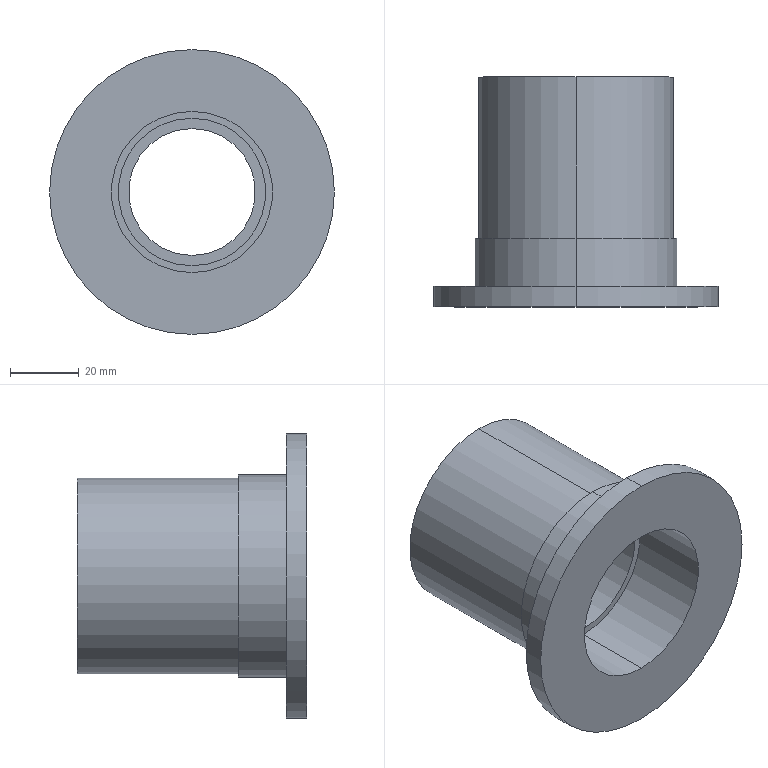Part | SolidWorks | features ICE 1, Revolution 1 | 1 solid | 24 faces | box 83 x 67 x 83 mm | volume 83007 mm3 | cylinder 16 | plane 8 | commonest cylinder face diameters 47 x4 37 x2 43 x2 49 x2 57 x2 59 x2
STEP:
#1=CARTESIAN_POINT('',(0.,67.,24.5));
#2=VERTEX_POINT('',#1);
#3=CARTESIAN_POINT('',(0.,67.,-24.5));
#4=VERTEX_POINT('',#3);
#5=CARTESIAN_POINT('',(0.,67.,0.));
#6=DIRECTION('',(0.,-1.,0.));
#7=DIRECTION('',(0.,0.,-1.));
#8=AXIS2_PLACEMENT_3D('',#5,#6,#7);
#9=CIRCLE('',#8,24.5);
#10=EDGE_CURVE('',#2,#4,#9,.T.);
#11=ORIENTED_EDGE('',*,*,#10,.F.);
#12=CARTESIAN_POINT('',(0.,57.,24.5));
#13=VERTEX_POINT('',#12);
#14=CARTESIAN_POINT('',(0.,0.,24.5));
#15=DIRECTION('',(0.,-1.,0.));
#16=VECTOR('',#15,1000.);
#17=LINE('',#14,#16);
#18=EDGE_CURVE('',#2,#13,#17,.T.);
#19=ORIENTED_EDGE('',*,*,#18,.T.);
#20=CARTESIAN_POINT('',(0.,57.,-24.5));
#21=VERTEX_POINT('',#20);
#22=CARTESIAN_POINT('',(0.,57.,0.));
#23=DIRECTION('',(0.,-1.,0.));
#24=DIRECTION('',(0.,0.,-1.));
#25=AXIS2_PLACEMENT_3D('',#22,#23,#24);
#26=CIRCLE('',#25,24.5);
#27=EDGE_CURVE('',#13,#21,#26,.T.);
#28=ORIENTED_EDGE('',*,*,#27,.T.);
#29=CARTESIAN_POINT('',(0.,0.,-24.5));
#30=DIRECTION('',(0.,-1.,0.));
#31=VECTOR('',#30,1000.);
#32=LINE('',#29,#31);
#33=EDGE_CURVE('',#4,#21,#32,.T.);
#34=ORIENTED_EDGE('',*,*,#33,.F.);
#35=EDGE_LOOP('',(#11,#19,#28,#34));
#36=FACE_OUTER_BOUND('',#35,.T.);
#37=CARTESIAN_POINT('',(0.,0.,0.));
#38=DIRECTION('',(0.,-1.,0.));
#39=DIRECTION('',(0.,0.,-1.));
#40=AXIS2_PLACEMENT_3D('',#37,#38,#39);
#41=CYLINDRICAL_SURFACE('',#40,24.5);
#42=ADVANCED_FACE('',(#36),#41,.F.);
#43=CARTESIAN_POINT('',(0.,67.,-28.5));
#44=VERTEX_POINT('',#43);
#45=CARTESIAN_POINT('',(0.,67.,28.5));
#46=VERTEX_POINT('',#45);
#47=CARTESIAN_POINT('',(0.,67.,0.));
#48=DIRECTION('',(0.,-1.,0.));
#49=DIRECTION('',(0.,0.,-1.));
#50=AXIS2_PLACEMENT_3D('',#47,#48,#49);
#51=CIRCLE('',#50,28.5);
#52=EDGE_CURVE('',#44,#46,#51,.T.);
#53=ORIENTED_EDGE('',*,*,#52,.T.);
#54=CARTESIAN_POINT('',(0.,20.,28.5));
#55=VERTEX_POINT('',#54);
#56=CARTESIAN_POINT('',(0.,0.,28.5));
#57=DIRECTION('',(0.,-1.,0.));
#58=VECTOR('',#57,1000.);
#59=LINE('',#56,#58);
#60=EDGE_CURVE('',#46,#55,#59,.T.);
#61=ORIENTED_EDGE('',*,*,#60,.T.);
#62=CARTESIAN_POINT('',(0.,20.,-28.5));
#63=VERTEX_POINT('',#62);
#64=CARTESIAN_POINT('',(0.,20.,0.));
#65=DIRECTION('',(0.,-1.,0.));
#66=DIRECTION('',(0.,0.,-1.));
#67=AXIS2_PLACEMENT_3D('',#64,#65,#66);
#68=CIRCLE('',#67,28.5);
#69=EDGE_CURVE('',#63,#55,#68,.T.);
#70=ORIENTED_EDGE('',*,*,#69,.F.);
#71=CARTESIAN_POINT('',(0.,0.,-28.5));
#72=DIRECTION('',(0.,-1.,0.));
#73=VECTOR('',#72,1000.);
#74=LINE('',#71,#73);
#75=EDGE_CURVE('',#44,#63,#74,.T.);
#76=ORIENTED_EDGE('',*,*,#75,.F.);
#77=EDGE_LOOP('',(#53,#61,#70,#76));
#78=FACE_OUTER_BOUND('',#77,.T.);
#79=CARTESIAN_POINT('',(0.,0.,0.));
#80=DIRECTION('',(0.,-1.,0.));
#81=DIRECTION('',(0.,0.,-1.));
#82=AXIS2_PLACEMENT_3D('',#79,#80,#81);
#83=CYLINDRICAL_SURFACE('',#82,28.5);
#84=ADVANCED_FACE('',(#78),#83,.T.);
#85=CARTESIAN_POINT('',(0.,20.,-29.5));
#86=VERTEX_POINT('',#85);
#87=CARTESIAN_POINT('',(0.,20.,29.5));
#88=VERTEX_POINT('',#87);
#89=CARTESIAN_POINT('',(0.,20.,0.));
#90=DIRECTION('',(0.,-1.,0.));
#91=DIRECTION('',(0.,0.,-1.));
#92=AXIS2_PLACEMENT_3D('',#89,#90,#91);
#93=CIRCLE('',#92,29.5);
#94=EDGE_CURVE('',#86,#88,#93,.T.);
#95=ORIENTED_EDGE('',*,*,#94,.T.);
#96=CARTESIAN_POINT('',(0.,6.,29.5));
#97=VERTEX_POINT('',#96);
#98=CARTESIAN_POINT('',(0.,0.,29.5));
#99=DIRECTION('',(0.,-1.,0.));
#100=VECTOR('',#99,1000.);
#101=LINE('',#98,#100);
#102=EDGE_CURVE('',#88,#97,#101,.T.);
#103=ORIENTED_EDGE('',*,*,#102,.T.);
#104=CARTESIAN_POINT('',(0.,6.,-29.5));
#105=VERTEX_POINT('',#104);
#106=CARTESIAN_POINT('',(0.,6.,0.));
#107=DIRECTION('',(0.,-1.,0.));
#108=DIRECTION('',(0.,0.,-1.));
#109=AXIS2_PLACEMENT_3D('',#106,#107,#108);
#110=CIRCLE('',#109,29.5);
#111=EDGE_CURVE('',#105,#97,#110,.T.);
#112=ORIENTED_EDGE('',*,*,#111,.F.);
#113=CARTESIAN_POINT('',(0.,0.,-29.5));
#114=DIRECTION('',(0.,-1.,0.));
#115=VECTOR('',#114,1000.);
#116=LINE('',#113,#115);
#117=EDGE_CURVE('',#86,#105,#116,.T.);
#118=ORIENTED_EDGE('',*,*,#117,.F.);
#119=EDGE_LOOP('',(#95,#103,#112,#118));
#120=FACE_OUTER_BOUND('',#119,.T.);
#121=CARTESIAN_POINT('',(0.,0.,0.));
#122=DIRECTION('',(0.,-1.,0.));
#123=DIRECTION('',(0.,0.,-1.));
#124=AXIS2_PLACEMENT_3D('',#121,#122,#123);
#125=CYLINDRICAL_SURFACE('',#124,29.5);
#126=ADVANCED_FACE('',(#120),#125,.T.);
#127=CARTESIAN_POINT('',(0.,6.,-41.5));
#128=VERTEX_POINT('',#127);
#129=CARTESIAN_POINT('',(0.,6.,41.5));
#130=VERTEX_POINT('',#129);
#131=CARTESIAN_POINT('',(0.,6.,0.));
#132=DIRECTION('',(0.,-1.,0.));
#133=DIRECTION('',(0.,0.,-1.));
#134=AXIS2_PLACEMENT_3D('',#131,#132,#133);
#135=CIRCLE('',#134,41.5);
#136=EDGE_CURVE('',#128,#130,#135,.T.);
#137=ORIENTED_EDGE('',*,*,#136,.T.);
#138=CARTESIAN_POINT('',(0.,0.,41.5));
#139=VERTEX_POINT('',#138);
#140=CARTESIAN_POINT('',(0.,0.,41.5));
#141=DIRECTION('',(0.,-1.,0.));
#142=VECTOR('',#141,1000.);
#143=LINE('',#140,#142);
#144=EDGE_CURVE('',#130,#139,#143,.T.);
#145=ORIENTED_EDGE('',*,*,#144,.T.);
#146=CARTESIAN_POINT('',(0.,0.,-41.5));
#147=VERTEX_POINT('',#146);
#148=CARTESIAN_POINT('',(0.,0.,0.));
#149=DIRECTION('',(0.,-1.,0.));
#150=DIRECTION('',(0.,0.,-1.));
#151=AXIS2_PLACEMENT_3D('',#148,#149,#150);
#152=CIRCLE('',#151,41.5);
#153=EDGE_CURVE('',#147,#139,#152,.T.);
#154=ORIENTED_EDGE('',*,*,#153,.F.);
#155=CARTESIAN_POINT('',(0.,0.,-41.5));
#156=DIRECTION('',(0.,-1.,0.));
#157=VECTOR('',#156,1000.);
#158=LINE('',#155,#157);
#159=EDGE_CURVE('',#128,#147,#158,.T.);
#160=ORIENTED_EDGE('',*,*,#159,.F.);
#161=EDGE_LOOP('',(#137,#145,#154,#160));
#162=FACE_OUTER_BOUND('',#161,.T.);
#163=CARTESIAN_POINT('',(0.,0.,0.));
#164=DIRECTION('',(0.,-1.,0.));
#165=DIRECTION('',(0.,0.,-1.));
#166=AXIS2_PLACEMENT_3D('',#163,#164,#165);
#167=CYLINDRICAL_SURFACE('',#166,41.5);
#168=ADVANCED_FACE('',(#162),#167,.T.);
#169=CARTESIAN_POINT('',(0.,24.,23.5));
#170=VERTEX_POINT('',#169);
#171=CARTESIAN_POINT('',(0.,24.,-23.5));
#172=VERTEX_POINT('',#171);
#173=CARTESIAN_POINT('',(0.,24.,0.));
#174=DIRECTION('',(0.,-1.,0.));
#175=DIRECTION('',(0.,0.,-1.));
#176=AXIS2_PLACEMENT_3D('',#173,#174,#175);
#177=CIRCLE('',#176,23.5);
#178=EDGE_CURVE('',#170,#172,#177,.T.);
#179=ORIENTED_EDGE('',*,*,#178,.F.);
#180=CARTESIAN_POINT('',(0.,0.,23.5));
#181=VERTEX_POINT('',#180);
#182=CARTESIAN_POINT('',(0.,0.,23.5));
#183=DIRECTION('',(0.,-1.,0.));
#184=VECTOR('',#183,1000.);
#185=LINE('',#182,#184);
#186=EDGE_CURVE('',#170,#181,#185,.T.);
#187=ORIENTED_EDGE('',*,*,#186,.T.);
#188=CARTESIAN_POINT('',(0.,0.,-23.5));
#189=VERTEX_POINT('',#188);
#190=CARTESIAN_POINT('',(0.,0.,0.));
#191=DIRECTION('',(0.,-1.,0.));
#192=DIRECTION('',(0.,0.,-1.));
#193=AXIS2_PLACEMENT_3D('',#190,#191,#192);
#194=CIRCLE('',#193,23.5);
#195=EDGE_CURVE('',#181,#189,#194,.T.);
#196=ORIENTED_EDGE('',*,*,#195,.T.);
#197=CARTESIAN_POINT('',(0.,0.,-23.5));
#198=DIRECTION('',(0.,-1.,0.));
#199=VECTOR('',#198,1000.);
#200=LINE('',#197,#199);
#201=EDGE_CURVE('',#172,#189,#200,.T.);
#202=ORIENTED_EDGE('',*,*,#201,.F.);
#203=EDGE_LOOP('',(#179,#187,#196,#202));
#204=FACE_OUTER_BOUND('',#203,.T.);
#205=CARTESIAN_POINT('',(0.,0.,0.));
#206=DIRECTION('',(0.,-1.,0.));
#207=DIRECTION('',(0.,0.,-1.));
#208=AXIS2_PLACEMENT_3D('',#205,#206,#207);
#209=CYLINDRICAL_SURFACE('',#208,23.5);
#210=ADVANCED_FACE('',(#204),#209,.F.);
#211=CARTESIAN_POINT('',(0.,48.,21.5));
#212=VERTEX_POINT('',#211);
#213=CARTESIAN_POINT('',(0.,48.,-21.5));
#214=VERTEX_POINT('',#213);
#215=CARTESIAN_POINT('',(0.,48.,0.));
#216=DIRECTION('',(0.,-1.,0.));
#217=DIRECTION('',(0.,0.,-1.));
#218=AXIS2_PLACEMENT_3D('',#215,#216,#217);
#219=CIRCLE('',#218,21.5);
#220=EDGE_CURVE('',#212,#214,#219,.T.);
#221=ORIENTED_EDGE('',*,*,#220,.F.);
#222=CARTESIAN_POINT('',(0.,24.,21.5));
#223=VERTEX_POINT('',#222);
#224=CARTESIAN_POINT('',(0.,0.,21.5));
#225=DIRECTION('',(0.,-1.,0.));
#226=VECTOR('',#225,1000.);
#227=LINE('',#224,#226);
#228=EDGE_CURVE('',#212,#223,#227,.T.);
#229=ORIENTED_EDGE('',*,*,#228,.T.);
#230=CARTESIAN_POINT('',(0.,24.,-21.5));
#231=VERTEX_POINT('',#230);
#232=CARTESIAN_POINT('',(0.,24.,0.));
#233=DIRECTION('',(0.,-1.,0.));
#234=DIRECTION('',(0.,0.,-1.));
#235=AXIS2_PLACEMENT_3D('',#232,#233,#234);
#236=CIRCLE('',#235,21.5);
#237=EDGE_CURVE('',#223,#231,#236,.T.);
#238=ORIENTED_EDGE('',*,*,#237,.T.);
#239=CARTESIAN_POINT('',(0.,0.,-21.5));
#240=DIRECTION('',(0.,-1.,0.));
#241=VECTOR('',#240,1000.);
#242=LINE('',#239,#241);
#243=EDGE_CURVE('',#214,#231,#242,.T.);
#244=ORIENTED_EDGE('',*,*,#243,.F.);
#245=EDGE_LOOP('',(#221,#229,#238,#244));
#246=FACE_OUTER_BOUND('',#245,.T.);
#247=CARTESIAN_POINT('',(0.,0.,0.));
#248=DIRECTION('',(0.,-1.,0.));
#249=DIRECTION('',(0.,0.,-1.));
#250=AXIS2_PLACEMENT_3D('',#247,#248,#249);
#251=CYLINDRICAL_SURFACE('',#250,21.5);
#252=ADVANCED_FACE('',(#246),#251,.F.);
#253=CARTESIAN_POINT('',(0.,53.,18.5));
#254=VERTEX_POINT('',#253);
#255=CARTESIAN_POINT('',(0.,53.,-18.5));
#256=VERTEX_POINT('',#255);
#257=CARTESIAN_POINT('',(0.,53.,0.));
#258=DIRECTION('',(0.,-1.,0.));
#259=DIRECTION('',(0.,0.,-1.));
#260=AXIS2_PLACEMENT_3D('',#257,#258,#259);
#261=CIRCLE('',#260,18.5);
#262=EDGE_CURVE('',#254,#256,#261,.T.);
#263=ORIENTED_EDGE('',*,*,#262,.F.);
#264=CARTESIAN_POINT('',(0.,48.,18.5));
#265=VERTEX_POINT('',#264);
#266=CARTESIAN_POINT('',(0.,0.,18.5));
#267=DIRECTION('',(0.,-1.,0.));
#268=VECTOR('',#267,1000.);
#269=LINE('',#266,#268);
#270=EDGE_CURVE('',#254,#265,#269,.T.);
#271=ORIENTED_EDGE('',*,*,#270,.T.);
#272=CARTESIAN_POINT('',(0.,48.,-18.5));
#273=VERTEX_POINT('',#272);
#274=CARTESIAN_POINT('',(0.,48.,0.));
#275=DIRECTION('',(0.,-1.,0.));
#276=DIRECTION('',(0.,0.,-1.));
#277=AXIS2_PLACEMENT_3D('',#274,#275,#276);
#278=CIRCLE('',#277,18.5);
#279=EDGE_CURVE('',#265,#273,#278,.T.);
#280=ORIENTED_EDGE('',*,*,#279,.T.);
#281=CARTESIAN_POINT('',(0.,0.,-18.5));
#282=DIRECTION('',(0.,-1.,0.));
#283=VECTOR('',#282,1000.);
#284=LINE('',#281,#283);
#285=EDGE_CURVE('',#256,#273,#284,.T.);
#286=ORIENTED_EDGE('',*,*,#285,.F.);
#287=EDGE_LOOP('',(#263,#271,#280,#286));
#288=FACE_OUTER_BOUND('',#287,.T.);
#289=CARTESIAN_POINT('',(0.,0.,0.));
#290=DIRECTION('',(0.,-1.,0.));
#291=DIRECTION('',(0.,0.,-1.));
#292=AXIS2_PLACEMENT_3D('',#289,#290,#291);
#293=CYLINDRICAL_SURFACE('',#292,18.5);
#294=ADVANCED_FACE('',(#288),#293,.F.);
#295=CARTESIAN_POINT('',(0.,57.,23.5));
#296=VERTEX_POINT('',#295);
#297=CARTESIAN_POINT('',(0.,57.,-23.5));
#298=VERTEX_POINT('',#297);
#299=CARTESIAN_POINT('',(0.,57.,0.));
#300=DIRECTION('',(0.,-1.,0.));
#301=DIRECTION('',(0.,0.,-1.));
#302=AXIS2_PLACEMENT_3D('',#299,#300,#301);
#303=CIRCLE('',#302,23.5);
#304=EDGE_CURVE('',#296,#298,#303,.T.);
#305=ORIENTED_EDGE('',*,*,#304,.F.);
#306=CARTESIAN_POINT('',(0.,53.,23.5));
#307=VERTEX_POINT('',#306);
#308=CARTESIAN_POINT('',(0.,0.,23.5));
#309=DIRECTION('',(0.,-1.,0.));
#310=VECTOR('',#309,1000.);
#311=LINE('',#308,#310);
#312=EDGE_CURVE('',#296,#307,#311,.T.);
#313=ORIENTED_EDGE('',*,*,#312,.T.);
#314=CARTESIAN_POINT('',(0.,53.,-23.5));
#315=VERTEX_POINT('',#314);
#316=CARTESIAN_POINT('',(0.,53.,0.));
#317=DIRECTION('',(0.,-1.,0.));
#318=DIRECTION('',(0.,0.,-1.));
#319=AXIS2_PLACEMENT_3D('',#316,#317,#318);
#320=CIRCLE('',#319,23.5);
#321=EDGE_CURVE('',#307,#315,#320,.T.);
#322=ORIENTED_EDGE('',*,*,#321,.T.);
#323=CARTESIAN_POINT('',(0.,0.,-23.5));
#324=DIRECTION('',(0.,-1.,0.));
#325=VECTOR('',#324,1000.);
#326=LINE('',#323,#325);
#327=EDGE_CURVE('',#298,#315,#326,.T.);
#328=ORIENTED_EDGE('',*,*,#327,.F.);
#329=EDGE_LOOP('',(#305,#313,#322,#328));
#330=FACE_OUTER_BOUND('',#329,.T.);
#331=CARTESIAN_POINT('',(0.,0.,0.));
#332=DIRECTION('',(0.,-1.,0.));
#333=DIRECTION('',(0.,0.,-1.));
#334=AXIS2_PLACEMENT_3D('',#331,#332,#333);
#335=CYLINDRICAL_SURFACE('',#334,23.5);
#336=ADVANCED_FACE('',(#330),#335,.F.);
#337=CARTESIAN_POINT('',(0.,57.,0.));
#338=DIRECTION('',(0.,-1.,0.));
#339=DIRECTION('',(0.,0.,-1.));
#340=AXIS2_PLACEMENT_3D('',#337,#338,#339);
#341=CIRCLE('',#340,24.5);
#342=EDGE_CURVE('',#21,#13,#341,.T.);
#343=ORIENTED_EDGE('',*,*,#342,.F.);
#344=ORIENTED_EDGE('',*,*,#27,.F.);
#345=EDGE_LOOP('',(#343,#344));
#346=FACE_OUTER_BOUND('',#345,.T.);
#347=CARTESIAN_POINT('',(0.,57.,0.));
#348=DIRECTION('',(0.,-1.,0.));
#349=DIRECTION('',(0.,0.,-1.));
#350=AXIS2_PLACEMENT_3D('',#347,#348,#349);
#351=CIRCLE('',#350,23.5);
#352=EDGE_CURVE('',#298,#296,#351,.T.);
#353=ORIENTED_EDGE('',*,*,#352,.T.);
#354=ORIENTED_EDGE('',*,*,#304,.T.);
#355=EDGE_LOOP('',(#353,#354));
#356=FACE_BOUND('',#355,.T.);
#357=CARTESIAN_POINT('',(-23.5,57.,0.));
#358=DIRECTION('',(0.,-1.,0.));
#359=DIRECTION('',(0.,0.,-1.));
#360=AXIS2_PLACEMENT_3D('',#357,#358,#359);
#361=PLANE('',#360);
#362=ADVANCED_FACE('',(#346,#356),#361,.F.);
#363=ORIENTED_EDGE('',*,*,#312,.F.);
#364=ORIENTED_EDGE('',*,*,#352,.F.);
#365=ORIENTED_EDGE('',*,*,#327,.T.);
#366=CARTESIAN_POINT('',(0.,53.,0.));
#367=DIRECTION('',(0.,-1.,0.));
#368=DIRECTION('',(0.,0.,-1.));
#369=AXIS2_PLACEMENT_3D('',#366,#367,#368);
#370=CIRCLE('',#369,23.5);
#371=EDGE_CURVE('',#315,#307,#370,.T.);
#372=ORIENTED_EDGE('',*,*,#371,.T.);
#373=EDGE_LOOP('',(#363,#364,#365,#372));
#374=FACE_OUTER_BOUND('',#373,.T.);
#375=CARTESIAN_POINT('',(0.,0.,0.));
#376=DIRECTION('',(0.,-1.,0.));
#377=DIRECTION('',(0.,0.,-1.));
#378=AXIS2_PLACEMENT_3D('',#375,#376,#377);
#379=CYLINDRICAL_SURFACE('',#378,23.5);
#380=ADVANCED_FACE('',(#374),#379,.F.);
#381=ORIENTED_EDGE('',*,*,#371,.F.);
#382=ORIENTED_EDGE('',*,*,#321,.F.);
#383=EDGE_LOOP('',(#381,#382));
#384=FACE_OUTER_BOUND('',#383,.T.);
#385=CARTESIAN_POINT('',(0.,53.,0.));
#386=DIRECTION('',(0.,-1.,0.));
#387=DIRECTION('',(0.,0.,-1.));
#388=AXIS2_PLACEMENT_3D('',#385,#386,#387);
#389=CIRCLE('',#388,18.5);
#390=EDGE_CURVE('',#256,#254,#389,.T.);
#391=ORIENTED_EDGE('',*,*,#390,.T.);
#392=ORIENTED_EDGE('',*,*,#262,.T.);
#393=EDGE_LOOP('',(#391,#392));
#394=FACE_BOUND('',#393,.T.);
#395=CARTESIAN_POINT('',(-23.5,53.,0.));
#396=DIRECTION('',(0.,-1.,0.));
#397=DIRECTION('',(0.,0.,-1.));
#398=AXIS2_PLACEMENT_3D('',#395,#396,#397);
#399=PLANE('',#398);
#400=ADVANCED_FACE('',(#384,#394),#399,.F.);
#401=ORIENTED_EDGE('',*,*,#270,.F.);
#402=ORIENTED_EDGE('',*,*,#390,.F.);
#403=ORIENTED_EDGE('',*,*,#285,.T.);
#404=CARTESIAN_POINT('',(0.,48.,0.));
#405=DIRECTION('',(0.,-1.,0.));
#406=DIRECTION('',(0.,0.,-1.));
#407=AXIS2_PLACEMENT_3D('',#404,#405,#406);
#408=CIRCLE('',#407,18.5);
#409=EDGE_CURVE('',#273,#265,#408,.T.);
#410=ORIENTED_EDGE('',*,*,#409,.T.);
#411=EDGE_LOOP('',(#401,#402,#403,#410));
#412=FACE_OUTER_BOUND('',#411,.T.);
#413=CARTESIAN_POINT('',(0.,0.,0.));
#414=DIRECTION('',(0.,-1.,0.));
#415=DIRECTION('',(0.,0.,-1.));
#416=AXIS2_PLACEMENT_3D('',#413,#414,#415);
#417=CYLINDRICAL_SURFACE('',#416,18.5);
#418=ADVANCED_FACE('',(#412),#417,.F.);
#419=ORIENTED_EDGE('',*,*,#409,.F.);
#420=ORIENTED_EDGE('',*,*,#279,.F.);
#421=EDGE_LOOP('',(#419,#420));
#422=FACE_BOUND('',#421,.T.);
#423=CARTESIAN_POINT('',(0.,48.,0.));
#424=DIRECTION('',(0.,-1.,0.));
#425=DIRECTION('',(0.,0.,-1.));
#426=AXIS2_PLACEMENT_3D('',#423,#424,#425);
#427=CIRCLE('',#426,21.5);
#428=EDGE_CURVE('',#214,#212,#427,.T.);
#429=ORIENTED_EDGE('',*,*,#428,.T.);
#430=ORIENTED_EDGE('',*,*,#220,.T.);
#431=EDGE_LOOP('',(#429,#430));
#432=FACE_OUTER_BOUND('',#431,.T.);
#433=CARTESIAN_POINT('',(-18.5,48.,0.));
#434=DIRECTION('',(0.,1.,0.));
#435=DIRECTION('',(0.,0.,1.));
#436=AXIS2_PLACEMENT_3D('',#433,#434,#435);
#437=PLANE('',#436);
#438=ADVANCED_FACE('',(#422,#432),#437,.F.);
#439=ORIENTED_EDGE('',*,*,#228,.F.);
#440=ORIENTED_EDGE('',*,*,#428,.F.);
#441=ORIENTED_EDGE('',*,*,#243,.T.);
#442=CARTESIAN_POINT('',(0.,24.,0.));
#443=DIRECTION('',(0.,-1.,0.));
#444=DIRECTION('',(0.,0.,-1.));
#445=AXIS2_PLACEMENT_3D('',#442,#443,#444);
#446=CIRCLE('',#445,21.5);
#447=EDGE_CURVE('',#231,#223,#446,.T.);
#448=ORIENTED_EDGE('',*,*,#447,.T.);
#449=EDGE_LOOP('',(#439,#440,#441,#448));
#450=FACE_OUTER_BOUND('',#449,.T.);
#451=CARTESIAN_POINT('',(0.,0.,0.));
#452=DIRECTION('',(0.,-1.,0.));
#453=DIRECTION('',(0.,0.,-1.));
#454=AXIS2_PLACEMENT_3D('',#451,#452,#453);
#455=CYLINDRICAL_SURFACE('',#454,21.5);
#456=ADVANCED_FACE('',(#450),#455,.F.);
#457=ORIENTED_EDGE('',*,*,#447,.F.);
#458=ORIENTED_EDGE('',*,*,#237,.F.);
#459=EDGE_LOOP('',(#457,#458));
#460=FACE_BOUND('',#459,.T.);
#461=CARTESIAN_POINT('',(0.,24.,0.));
#462=DIRECTION('',(0.,-1.,0.));
#463=DIRECTION('',(0.,0.,-1.));
#464=AXIS2_PLACEMENT_3D('',#461,#462,#463);
#465=CIRCLE('',#464,23.5);
#466=EDGE_CURVE('',#172,#170,#465,.T.);
#467=ORIENTED_EDGE('',*,*,#466,.T.);
#468=ORIENTED_EDGE('',*,*,#178,.T.);
#469=EDGE_LOOP('',(#467,#468));
#470=FACE_OUTER_BOUND('',#469,.T.);
#471=CARTESIAN_POINT('',(-21.5,24.,0.));
#472=DIRECTION('',(0.,1.,0.));
#473=DIRECTION('',(0.,0.,1.));
#474=AXIS2_PLACEMENT_3D('',#471,#472,#473);
#475=PLANE('',#474);
#476=ADVANCED_FACE('',(#460,#470),#475,.F.);
#477=ORIENTED_EDGE('',*,*,#186,.F.);
#478=ORIENTED_EDGE('',*,*,#466,.F.);
#479=ORIENTED_EDGE('',*,*,#201,.T.);
#480=CARTESIAN_POINT('',(0.,0.,0.));
#481=DIRECTION('',(0.,-1.,0.));
#482=DIRECTION('',(0.,0.,-1.));
#483=AXIS2_PLACEMENT_3D('',#480,#481,#482);
#484=CIRCLE('',#483,23.5);
#485=EDGE_CURVE('',#189,#181,#484,.T.);
#486=ORIENTED_EDGE('',*,*,#485,.T.);
#487=EDGE_LOOP('',(#477,#478,#479,#486));
#488=FACE_OUTER_BOUND('',#487,.T.);
#489=CARTESIAN_POINT('',(0.,0.,0.));
#490=DIRECTION('',(0.,-1.,0.));
#491=DIRECTION('',(0.,0.,-1.));
#492=AXIS2_PLACEMENT_3D('',#489,#490,#491);
#493=CYLINDRICAL_SURFACE('',#492,23.5);
#494=ADVANCED_FACE('',(#488),#493,.F.);
#495=ORIENTED_EDGE('',*,*,#485,.F.);
#496=ORIENTED_EDGE('',*,*,#195,.F.);
#497=EDGE_LOOP('',(#495,#496));
#498=FACE_BOUND('',#497,.T.);
#499=ORIENTED_EDGE('',*,*,#153,.T.);
#500=CARTESIAN_POINT('',(0.,0.,0.));
#501=DIRECTION('',(0.,-1.,0.));
#502=DIRECTION('',(0.,0.,-1.));
#503=AXIS2_PLACEMENT_3D('',#500,#501,#502);
#504=CIRCLE('',#503,41.5);
#505=EDGE_CURVE('',#139,#147,#504,.T.);
#506=ORIENTED_EDGE('',*,*,#505,.T.);
#507=EDGE_LOOP('',(#499,#506));
#508=FACE_OUTER_BOUND('',#507,.T.);
#509=CARTESIAN_POINT('',(-23.5,0.,0.));
#510=DIRECTION('',(0.,1.,0.));
#511=DIRECTION('',(0.,0.,1.));
#512=AXIS2_PLACEMENT_3D('',#509,#510,#511);
#513=PLANE('',#512);
#514=ADVANCED_FACE('',(#498,#508),#513,.F.);
#515=ORIENTED_EDGE('',*,*,#144,.F.);
#516=CARTESIAN_POINT('',(0.,6.,0.));
#517=DIRECTION('',(0.,-1.,0.));
#518=DIRECTION('',(0.,0.,-1.));
#519=AXIS2_PLACEMENT_3D('',#516,#517,#518);
#520=CIRCLE('',#519,41.5);
#521=EDGE_CURVE('',#130,#128,#520,.T.);
#522=ORIENTED_EDGE('',*,*,#521,.T.);
#523=ORIENTED_EDGE('',*,*,#159,.T.);
#524=ORIENTED_EDGE('',*,*,#505,.F.);
#525=EDGE_LOOP('',(#515,#522,#523,#524));
#526=FACE_OUTER_BOUND('',#525,.T.);
#527=CARTESIAN_POINT('',(0.,0.,0.));
#528=DIRECTION('',(0.,-1.,0.));
#529=DIRECTION('',(0.,0.,-1.));
#530=AXIS2_PLACEMENT_3D('',#527,#528,#529);
#531=CYLINDRICAL_SURFACE('',#530,41.5);
#532=ADVANCED_FACE('',(#526),#531,.T.);
#533=ORIENTED_EDGE('',*,*,#136,.F.);
#534=ORIENTED_EDGE('',*,*,#521,.F.);
#535=EDGE_LOOP('',(#533,#534));
#536=FACE_OUTER_BOUND('',#535,.T.);
#537=ORIENTED_EDGE('',*,*,#111,.T.);
#538=CARTESIAN_POINT('',(0.,6.,0.));
#539=DIRECTION('',(0.,-1.,0.));
#540=DIRECTION('',(0.,0.,-1.));
#541=AXIS2_PLACEMENT_3D('',#538,#539,#540);
#542=CIRCLE('',#541,29.5);
#543=EDGE_CURVE('',#97,#105,#542,.T.);
#544=ORIENTED_EDGE('',*,*,#543,.T.);
#545=EDGE_LOOP('',(#537,#544));
#546=FACE_BOUND('',#545,.T.);
#547=CARTESIAN_POINT('',(-29.5,6.,0.));
#548=DIRECTION('',(0.,-1.,0.));
#549=DIRECTION('',(0.,0.,-1.));
#550=AXIS2_PLACEMENT_3D('',#547,#548,#549);
#551=PLANE('',#550);
#552=ADVANCED_FACE('',(#536,#546),#551,.F.);
#553=ORIENTED_EDGE('',*,*,#102,.F.);
#554=CARTESIAN_POINT('',(0.,20.,0.));
#555=DIRECTION('',(0.,-1.,0.));
#556=DIRECTION('',(0.,0.,-1.));
#557=AXIS2_PLACEMENT_3D('',#554,#555,#556);
#558=CIRCLE('',#557,29.5);
#559=EDGE_CURVE('',#88,#86,#558,.T.);
#560=ORIENTED_EDGE('',*,*,#559,.T.);
#561=ORIENTED_EDGE('',*,*,#117,.T.);
#562=ORIENTED_EDGE('',*,*,#543,.F.);
#563=EDGE_LOOP('',(#553,#560,#561,#562));
#564=FACE_OUTER_BOUND('',#563,.T.);
#565=CARTESIAN_POINT('',(0.,0.,0.));
#566=DIRECTION('',(0.,-1.,0.));
#567=DIRECTION('',(0.,0.,-1.));
#568=AXIS2_PLACEMENT_3D('',#565,#566,#567);
#569=CYLINDRICAL_SURFACE('',#568,29.5);
#570=ADVANCED_FACE('',(#564),#569,.T.);
#571=ORIENTED_EDGE('',*,*,#94,.F.);
#572=ORIENTED_EDGE('',*,*,#559,.F.);
#573=EDGE_LOOP('',(#571,#572));
#574=FACE_OUTER_BOUND('',#573,.T.);
#575=ORIENTED_EDGE('',*,*,#69,.T.);
#576=CARTESIAN_POINT('',(0.,20.,0.));
#577=DIRECTION('',(0.,-1.,0.));
#578=DIRECTION('',(0.,0.,-1.));
#579=AXIS2_PLACEMENT_3D('',#576,#577,#578);
#580=CIRCLE('',#579,28.5);
#581=EDGE_CURVE('',#55,#63,#580,.T.);
#582=ORIENTED_EDGE('',*,*,#581,.T.);
#583=EDGE_LOOP('',(#575,#582));
#584=FACE_BOUND('',#583,.T.);
#585=CARTESIAN_POINT('',(-28.5,20.,0.));
#586=DIRECTION('',(0.,-1.,0.));
#587=DIRECTION('',(0.,0.,-1.));
#588=AXIS2_PLACEMENT_3D('',#585,#586,#587);
#589=PLANE('',#588);
#590=ADVANCED_FACE('',(#574,#584),#589,.F.);
#591=ORIENTED_EDGE('',*,*,#60,.F.);
#592=CARTESIAN_POINT('',(0.,67.,0.));
#593=DIRECTION('',(0.,-1.,0.));
#594=DIRECTION('',(0.,0.,-1.));
#595=AXIS2_PLACEMENT_3D('',#592,#593,#594);
#596=CIRCLE('',#595,28.5);
#597=EDGE_CURVE('',#46,#44,#596,.T.);
#598=ORIENTED_EDGE('',*,*,#597,.T.);
#599=ORIENTED_EDGE('',*,*,#75,.T.);
#600=ORIENTED_EDGE('',*,*,#581,.F.);
#601=EDGE_LOOP('',(#591,#598,#599,#600));
#602=FACE_OUTER_BOUND('',#601,.T.);
#603=CARTESIAN_POINT('',(0.,0.,0.));
#604=DIRECTION('',(0.,-1.,0.));
#605=DIRECTION('',(0.,0.,-1.));
#606=AXIS2_PLACEMENT_3D('',#603,#604,#605);
#607=CYLINDRICAL_SURFACE('',#606,28.5);
#608=ADVANCED_FACE('',(#602),#607,.T.);
#609=ORIENTED_EDGE('',*,*,#52,.F.);
#610=ORIENTED_EDGE('',*,*,#597,.F.);
#611=EDGE_LOOP('',(#609,#610));
#612=FACE_OUTER_BOUND('',#611,.T.);
#613=CARTESIAN_POINT('',(0.,67.,0.));
#614=DIRECTION('',(0.,-1.,0.));
#615=DIRECTION('',(0.,0.,-1.));
#616=AXIS2_PLACEMENT_3D('',#613,#614,#615);
#617=CIRCLE('',#616,24.5);
#618=EDGE_CURVE('',#4,#2,#617,.T.);
#619=ORIENTED_EDGE('',*,*,#618,.T.);
#620=ORIENTED_EDGE('',*,*,#10,.T.);
#621=EDGE_LOOP('',(#619,#620));
#622=FACE_BOUND('',#621,.T.);
#623=CARTESIAN_POINT('',(-24.5,67.,0.));
#624=DIRECTION('',(0.,-1.,0.));
#625=DIRECTION('',(0.,0.,-1.));
#626=AXIS2_PLACEMENT_3D('',#623,#624,#625);
#627=PLANE('',#626);
#628=ADVANCED_FACE('',(#612,#622),#627,.F.);
#629=ORIENTED_EDGE('',*,*,#18,.F.);
#630=ORIENTED_EDGE('',*,*,#618,.F.);
#631=ORIENTED_EDGE('',*,*,#33,.T.);
#632=ORIENTED_EDGE('',*,*,#342,.T.);
#633=EDGE_LOOP('',(#629,#630,#631,#632));
#634=FACE_OUTER_BOUND('',#633,.T.);
#635=CARTESIAN_POINT('',(0.,0.,0.));
#636=DIRECTION('',(0.,-1.,0.));
#637=DIRECTION('',(0.,0.,-1.));
#638=AXIS2_PLACEMENT_3D('',#635,#636,#637);
#639=CYLINDRICAL_SURFACE('',#638,24.5);
#640=ADVANCED_FACE('',(#634),#639,.F.);
#641=CLOSED_SHELL('',(#42,#84,#126,#168,#210,#252,#294,#336,#362,#380,#400,#418,#438,#456,#476,#494,#514,#532,#552,#570,#590,#608,#628,#640));
#642=MANIFOLD_SOLID_BREP('',#641);
#643=CARTESIAN_POINT('',(0.,0.,0.));
#644=DIRECTION('',(0.,0.,1.));
#645=DIRECTION('',(1.,0.,0.));
#646=AXIS2_PLACEMENT_3D('',#643,#644,#645);
#647=(LENGTH_UNIT()NAMED_UNIT(*)SI_UNIT(.MILLI.,.METRE.));
#648=UNCERTAINTY_MEASURE_WITH_UNIT(LENGTH_MEASURE(0.00001),#647,'','');
#649=(NAMED_UNIT(*)PLANE_ANGLE_UNIT()SI_UNIT($,.RADIAN.));
#650=(NAMED_UNIT(*)SI_UNIT($,.STERADIAN.)SOLID_ANGLE_UNIT());
#651=(GEOMETRIC_REPRESENTATION_CONTEXT(3)GLOBAL_UNCERTAINTY_ASSIGNED_CONTEXT((#648))GLOBAL_UNIT_ASSIGNED_CONTEXT((#647,#649,#650))REPRESENTATION_CONTEXT('',''));
#652=ADVANCED_BREP_SHAPE_REPRESENTATION('',(#642,#646),#651);